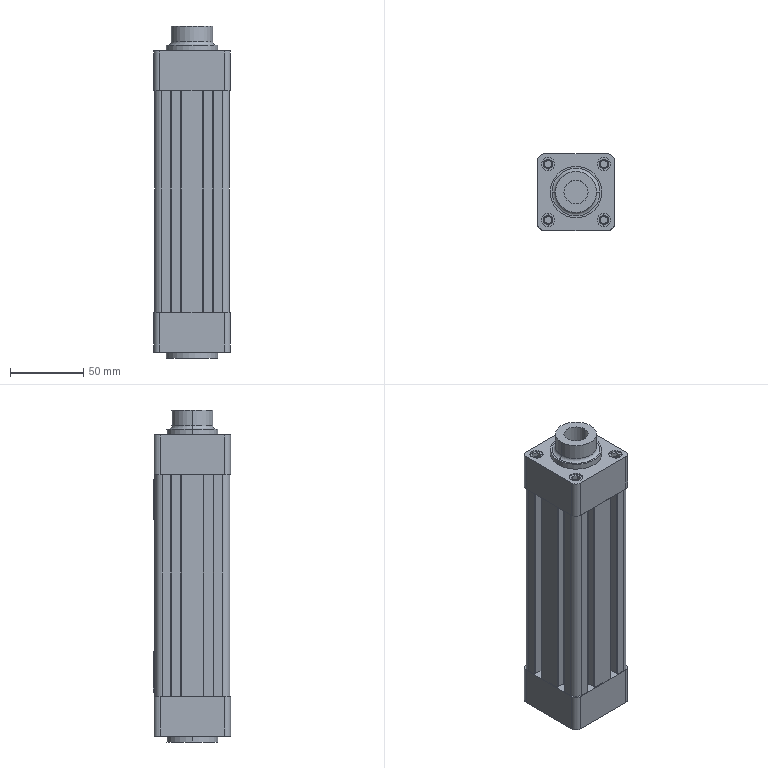Part | STEP file | 1 solid | 357 faces | box 52 x 52.5 x 226 mm | volume 470027 mm3 | plane 267 | cylinder 64 | cone 24 | torus 2 | commonest cylinder face diameters 4.773 x16 9 x16 8 x8 2.7 x4 7.8 x4 10 x4